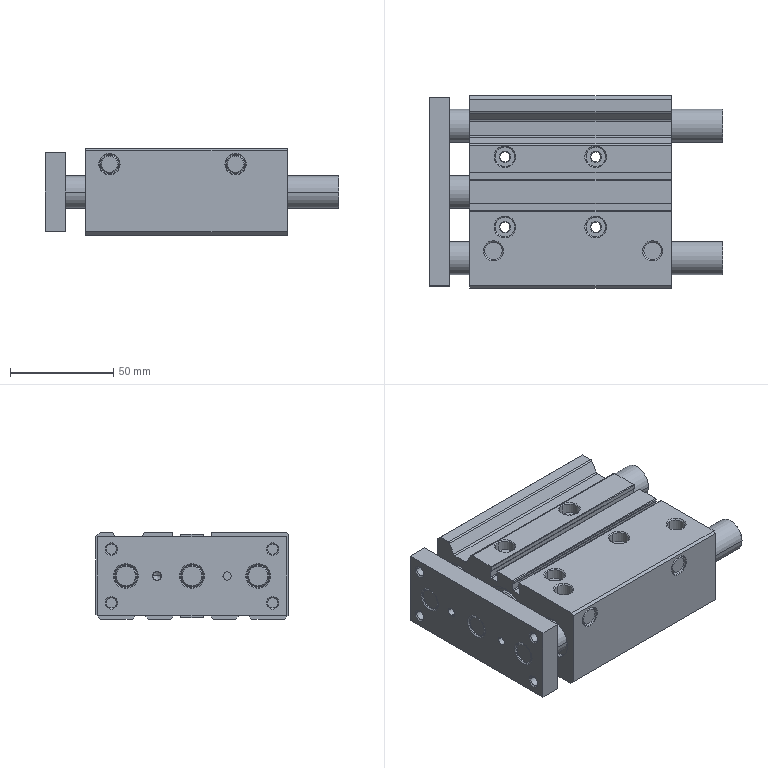Part | SolidWorks | 2 solids | 382 faces | box 142 x 93 x 42 mm | volume 365239 mm3 | cylinder 167 | plane 117 | cone 94 | spline 4 | commonest cylinder face diameters 0.8 x28 4.917 x24 4 x21 0.4 x12 16 x12 5.5 x8